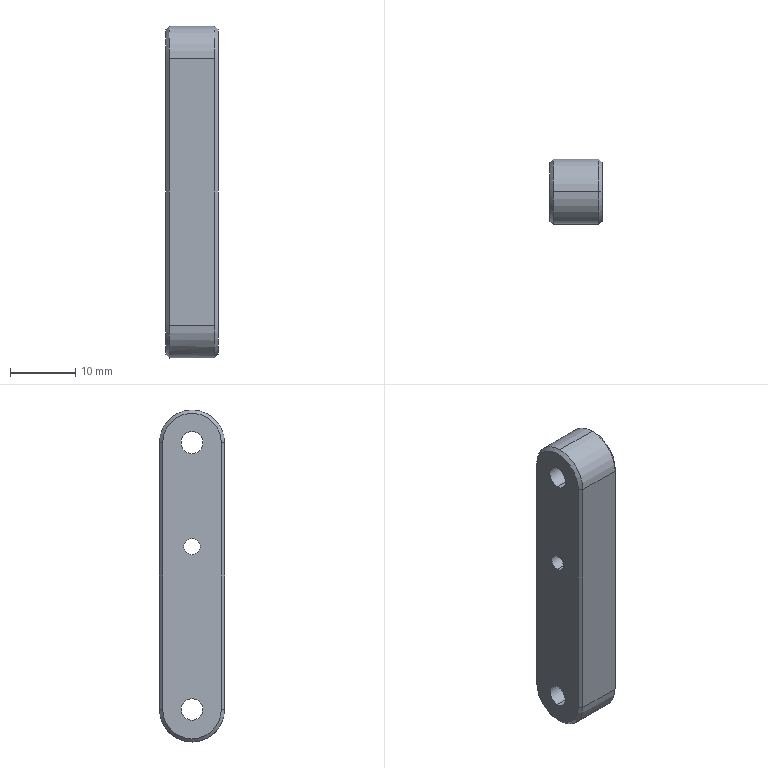Part | SolidWorks | features HoleWzd 3, Chamfer 1, Extrusion 1 | 1 solid | 26 faces | box 8 x 10 x 51 mm | volume 3618 mm3 | cylinder 11 | plane 9 | cone 6 | commonest cylinder face diameters 10 x3 2.5 x2 3.3 x2 3.4 x2 6.5 x2
STEP:
#1=CARTESIAN_POINT('',(4.,0.,25.));
#2=VERTEX_POINT('',#1);
#3=CARTESIAN_POINT('',(4.,-4.5,20.5));
#4=VERTEX_POINT('',#3);
#5=CARTESIAN_POINT('',(4.,0.,20.5));
#6=DIRECTION('',(1.,0.,0.));
#7=DIRECTION('',(0.,0.,-1.));
#8=AXIS2_PLACEMENT_3D('',#5,#6,#7);
#9=CIRCLE('',#8,4.5);
#10=EDGE_CURVE('',#2,#4,#9,.T.);
#11=ORIENTED_EDGE('',*,*,#10,.F.);
#12=CARTESIAN_POINT('',(3.5,0.,25.5));
#13=VERTEX_POINT('',#12);
#14=CARTESIAN_POINT('',(4.,0.,25.));
#15=DIRECTION('',(-0.7071,0.,0.7071));
#16=VECTOR('',#15,1000.);
#17=LINE('',#14,#16);
#18=EDGE_CURVE('',#2,#13,#17,.T.);
#19=ORIENTED_EDGE('',*,*,#18,.T.);
#20=CARTESIAN_POINT('',(3.5,-5.,20.5));
#21=VERTEX_POINT('',#20);
#22=CARTESIAN_POINT('',(3.5,0.,20.5));
#23=DIRECTION('',(-1.,0.,0.));
#24=DIRECTION('',(0.,0.,-1.));
#25=AXIS2_PLACEMENT_3D('',#22,#23,#24);
#26=CIRCLE('',#25,5.);
#27=EDGE_CURVE('',#21,#13,#26,.T.);
#28=ORIENTED_EDGE('',*,*,#27,.F.);
#29=CARTESIAN_POINT('',(3.5,-5.,20.5));
#30=DIRECTION('',(0.7071,0.7071,0.));
#31=VECTOR('',#30,1000.);
#32=LINE('',#29,#31);
#33=EDGE_CURVE('',#21,#4,#32,.T.);
#34=ORIENTED_EDGE('',*,*,#33,.T.);
#35=EDGE_LOOP('',(#11,#19,#28,#34));
#36=FACE_OUTER_BOUND('',#35,.T.);
#37=CARTESIAN_POINT('',(4.,0.,20.5));
#38=DIRECTION('',(-1.,0.,0.));
#39=DIRECTION('',(0.,0.,1.));
#40=AXIS2_PLACEMENT_3D('',#37,#38,#39);
#41=CONICAL_SURFACE('',#40,4.5,0.7854);
#42=ADVANCED_FACE('',(#36),#41,.T.);
#43=CARTESIAN_POINT('',(-4.,0.,-25.));
#44=VERTEX_POINT('',#43);
#45=CARTESIAN_POINT('',(-4.,-4.5,-20.5));
#46=VERTEX_POINT('',#45);
#47=CARTESIAN_POINT('',(-4.,0.,-20.5));
#48=DIRECTION('',(-1.,0.,0.));
#49=DIRECTION('',(0.,0.,-1.));
#50=AXIS2_PLACEMENT_3D('',#47,#48,#49);
#51=CIRCLE('',#50,4.5);
#52=EDGE_CURVE('',#44,#46,#51,.T.);
#53=ORIENTED_EDGE('',*,*,#52,.F.);
#54=CARTESIAN_POINT('',(-3.5,0.,-25.5));
#55=VERTEX_POINT('',#54);
#56=CARTESIAN_POINT('',(-3.5,0.,-25.5));
#57=DIRECTION('',(0.7071,0.,-0.7071));
#58=VECTOR('',#57,1000.);
#59=LINE('',#56,#58);
#60=EDGE_CURVE('',#44,#55,#59,.T.);
#61=ORIENTED_EDGE('',*,*,#60,.T.);
#62=CARTESIAN_POINT('',(-3.5,-5.,-20.5));
#63=VERTEX_POINT('',#62);
#64=CARTESIAN_POINT('',(-3.5,0.,-20.5));
#65=DIRECTION('',(1.,0.,0.));
#66=DIRECTION('',(0.,0.,-1.));
#67=AXIS2_PLACEMENT_3D('',#64,#65,#66);
#68=CIRCLE('',#67,5.);
#69=EDGE_CURVE('',#63,#55,#68,.T.);
#70=ORIENTED_EDGE('',*,*,#69,.F.);
#71=CARTESIAN_POINT('',(-3.5,-5.,-20.5));
#72=DIRECTION('',(-0.7071,0.7071,0.));
#73=VECTOR('',#72,1000.);
#74=LINE('',#71,#73);
#75=EDGE_CURVE('',#63,#46,#74,.T.);
#76=ORIENTED_EDGE('',*,*,#75,.T.);
#77=EDGE_LOOP('',(#53,#61,#70,#76));
#78=FACE_OUTER_BOUND('',#77,.T.);
#79=CARTESIAN_POINT('',(-3.5,0.,-20.5));
#80=DIRECTION('',(1.,0.,0.));
#81=DIRECTION('',(0.,0.,-1.));
#82=AXIS2_PLACEMENT_3D('',#79,#80,#81);
#83=CONICAL_SURFACE('',#82,5.,0.7854);
#84=ADVANCED_FACE('',(#78),#83,.T.);
#85=CARTESIAN_POINT('',(-4.,0.,-18.85));
#86=VERTEX_POINT('',#85);
#87=CARTESIAN_POINT('',(-4.,0.,-22.15));
#88=VERTEX_POINT('',#87);
#89=CARTESIAN_POINT('',(-4.,0.,-20.5));
#90=DIRECTION('',(1.,0.,0.));
#91=DIRECTION('',(0.,0.,-1.));
#92=AXIS2_PLACEMENT_3D('',#89,#90,#91);
#93=CIRCLE('',#92,1.65);
#94=EDGE_CURVE('',#86,#88,#93,.T.);
#95=ORIENTED_EDGE('',*,*,#94,.F.);
#96=CARTESIAN_POINT('',(4.,0.,-18.85));
#97=VERTEX_POINT('',#96);
#98=CARTESIAN_POINT('',(4.,0.,-18.85));
#99=DIRECTION('',(1.,0.,0.));
#100=VECTOR('',#99,1000.);
#101=LINE('',#98,#100);
#102=EDGE_CURVE('',#86,#97,#101,.T.);
#103=ORIENTED_EDGE('',*,*,#102,.T.);
#104=CARTESIAN_POINT('',(4.,0.,-22.15));
#105=VERTEX_POINT('',#104);
#106=CARTESIAN_POINT('',(4.,0.,-20.5));
#107=DIRECTION('',(1.,0.,0.));
#108=DIRECTION('',(0.,0.,-1.));
#109=AXIS2_PLACEMENT_3D('',#106,#107,#108);
#110=CIRCLE('',#109,1.65);
#111=EDGE_CURVE('',#97,#105,#110,.T.);
#112=ORIENTED_EDGE('',*,*,#111,.T.);
#113=CARTESIAN_POINT('',(4.,0.,-22.15));
#114=DIRECTION('',(1.,0.,0.));
#115=VECTOR('',#114,1000.);
#116=LINE('',#113,#115);
#117=EDGE_CURVE('',#88,#105,#116,.T.);
#118=ORIENTED_EDGE('',*,*,#117,.F.);
#119=EDGE_LOOP('',(#95,#103,#112,#118));
#120=FACE_OUTER_BOUND('',#119,.T.);
#121=CARTESIAN_POINT('',(4.,0.,-20.5));
#122=DIRECTION('',(1.,0.,0.));
#123=DIRECTION('',(0.,0.,-1.));
#124=AXIS2_PLACEMENT_3D('',#121,#122,#123);
#125=CYLINDRICAL_SURFACE('',#124,1.65);
#126=ADVANCED_FACE('',(#120),#125,.F.);
#127=CARTESIAN_POINT('',(-4.,0.,5.75));
#128=VERTEX_POINT('',#127);
#129=CARTESIAN_POINT('',(-4.,0.,3.25));
#130=VERTEX_POINT('',#129);
#131=CARTESIAN_POINT('',(-4.,0.,4.5));
#132=DIRECTION('',(1.,0.,0.));
#133=DIRECTION('',(0.,0.,-1.));
#134=AXIS2_PLACEMENT_3D('',#131,#132,#133);
#135=CIRCLE('',#134,1.25);
#136=EDGE_CURVE('',#128,#130,#135,.T.);
#137=ORIENTED_EDGE('',*,*,#136,.F.);
#138=CARTESIAN_POINT('',(4.,0.,5.75));
#139=VERTEX_POINT('',#138);
#140=CARTESIAN_POINT('',(4.,0.,5.75));
#141=DIRECTION('',(1.,0.,0.));
#142=VECTOR('',#141,1000.);
#143=LINE('',#140,#142);
#144=EDGE_CURVE('',#128,#139,#143,.T.);
#145=ORIENTED_EDGE('',*,*,#144,.T.);
#146=CARTESIAN_POINT('',(4.,0.,3.25));
#147=VERTEX_POINT('',#146);
#148=CARTESIAN_POINT('',(4.,0.,4.5));
#149=DIRECTION('',(1.,0.,0.));
#150=DIRECTION('',(0.,0.,-1.));
#151=AXIS2_PLACEMENT_3D('',#148,#149,#150);
#152=CIRCLE('',#151,1.25);
#153=EDGE_CURVE('',#139,#147,#152,.T.);
#154=ORIENTED_EDGE('',*,*,#153,.T.);
#155=CARTESIAN_POINT('',(4.,0.,3.25));
#156=DIRECTION('',(1.,0.,0.));
#157=VECTOR('',#156,1000.);
#158=LINE('',#155,#157);
#159=EDGE_CURVE('',#130,#147,#158,.T.);
#160=ORIENTED_EDGE('',*,*,#159,.F.);
#161=EDGE_LOOP('',(#137,#145,#154,#160));
#162=FACE_OUTER_BOUND('',#161,.T.);
#163=CARTESIAN_POINT('',(4.,0.,4.5));
#164=DIRECTION('',(1.,0.,0.));
#165=DIRECTION('',(0.,0.,-1.));
#166=AXIS2_PLACEMENT_3D('',#163,#164,#165);
#167=CYLINDRICAL_SURFACE('',#166,1.25);
#168=ADVANCED_FACE('',(#162),#167,.F.);
#169=CARTESIAN_POINT('',(0.6,0.,23.75));
#170=VERTEX_POINT('',#169);
#171=CARTESIAN_POINT('',(0.6,0.,17.25));
#172=VERTEX_POINT('',#171);
#173=CARTESIAN_POINT('',(0.6,0.,20.5));
#174=DIRECTION('',(1.,0.,0.));
#175=DIRECTION('',(0.,0.,-1.));
#176=AXIS2_PLACEMENT_3D('',#173,#174,#175);
#177=CIRCLE('',#176,3.25);
#178=EDGE_CURVE('',#170,#172,#177,.T.);
#179=ORIENTED_EDGE('',*,*,#178,.F.);
#180=CARTESIAN_POINT('',(4.,0.,23.75));
#181=VERTEX_POINT('',#180);
#182=CARTESIAN_POINT('',(4.,0.,23.75));
#183=DIRECTION('',(1.,0.,0.));
#184=VECTOR('',#183,1000.);
#185=LINE('',#182,#184);
#186=EDGE_CURVE('',#170,#181,#185,.T.);
#187=ORIENTED_EDGE('',*,*,#186,.T.);
#188=CARTESIAN_POINT('',(4.,0.,17.25));
#189=VERTEX_POINT('',#188);
#190=CARTESIAN_POINT('',(4.,0.,20.5));
#191=DIRECTION('',(1.,0.,0.));
#192=DIRECTION('',(0.,0.,-1.));
#193=AXIS2_PLACEMENT_3D('',#190,#191,#192);
#194=CIRCLE('',#193,3.25);
#195=EDGE_CURVE('',#181,#189,#194,.T.);
#196=ORIENTED_EDGE('',*,*,#195,.T.);
#197=CARTESIAN_POINT('',(4.,0.,17.25));
#198=DIRECTION('',(1.,0.,0.));
#199=VECTOR('',#198,1000.);
#200=LINE('',#197,#199);
#201=EDGE_CURVE('',#172,#189,#200,.T.);
#202=ORIENTED_EDGE('',*,*,#201,.F.);
#203=EDGE_LOOP('',(#179,#187,#196,#202));
#204=FACE_OUTER_BOUND('',#203,.T.);
#205=CARTESIAN_POINT('',(4.,0.,20.5));
#206=DIRECTION('',(1.,0.,0.));
#207=DIRECTION('',(0.,0.,-1.));
#208=AXIS2_PLACEMENT_3D('',#205,#206,#207);
#209=CYLINDRICAL_SURFACE('',#208,3.25);
#210=ADVANCED_FACE('',(#204),#209,.F.);
#211=CARTESIAN_POINT('',(-4.,0.,22.2));
#212=VERTEX_POINT('',#211);
#213=CARTESIAN_POINT('',(-4.,0.,18.8));
#214=VERTEX_POINT('',#213);
#215=CARTESIAN_POINT('',(-4.,0.,20.5));
#216=DIRECTION('',(1.,0.,0.));
#217=DIRECTION('',(0.,0.,-1.));
#218=AXIS2_PLACEMENT_3D('',#215,#216,#217);
#219=CIRCLE('',#218,1.7);
#220=EDGE_CURVE('',#212,#214,#219,.T.);
#221=ORIENTED_EDGE('',*,*,#220,.F.);
#222=CARTESIAN_POINT('',(0.6,0.,22.2));
#223=VERTEX_POINT('',#222);
#224=CARTESIAN_POINT('',(4.,0.,22.2));
#225=DIRECTION('',(1.,0.,0.));
#226=VECTOR('',#225,1000.);
#227=LINE('',#224,#226);
#228=EDGE_CURVE('',#212,#223,#227,.T.);
#229=ORIENTED_EDGE('',*,*,#228,.T.);
#230=CARTESIAN_POINT('',(0.6,0.,18.8));
#231=VERTEX_POINT('',#230);
#232=CARTESIAN_POINT('',(0.6,0.,20.5));
#233=DIRECTION('',(1.,0.,0.));
#234=DIRECTION('',(0.,0.,-1.));
#235=AXIS2_PLACEMENT_3D('',#232,#233,#234);
#236=CIRCLE('',#235,1.7);
#237=EDGE_CURVE('',#223,#231,#236,.T.);
#238=ORIENTED_EDGE('',*,*,#237,.T.);
#239=CARTESIAN_POINT('',(4.,0.,18.8));
#240=DIRECTION('',(1.,0.,0.));
#241=VECTOR('',#240,1000.);
#242=LINE('',#239,#241);
#243=EDGE_CURVE('',#214,#231,#242,.T.);
#244=ORIENTED_EDGE('',*,*,#243,.F.);
#245=EDGE_LOOP('',(#221,#229,#238,#244));
#246=FACE_OUTER_BOUND('',#245,.T.);
#247=CARTESIAN_POINT('',(4.,0.,20.5));
#248=DIRECTION('',(1.,0.,0.));
#249=DIRECTION('',(0.,0.,-1.));
#250=AXIS2_PLACEMENT_3D('',#247,#248,#249);
#251=CYLINDRICAL_SURFACE('',#250,1.7);
#252=ADVANCED_FACE('',(#246),#251,.F.);
#253=ORIENTED_EDGE('',*,*,#27,.T.);
#254=CARTESIAN_POINT('',(-3.5,0.,25.5));
#255=VERTEX_POINT('',#254);
#256=CARTESIAN_POINT('',(4.,0.,25.5));
#257=DIRECTION('',(-1.,0.,0.));
#258=VECTOR('',#257,1000.);
#259=LINE('',#256,#258);
#260=EDGE_CURVE('',#13,#255,#259,.T.);
#261=ORIENTED_EDGE('',*,*,#260,.T.);
#262=CARTESIAN_POINT('',(-3.5,-5.,20.5));
#263=VERTEX_POINT('',#262);
#264=CARTESIAN_POINT('',(-3.5,0.,20.5));
#265=DIRECTION('',(1.,0.,0.));
#266=DIRECTION('',(0.,0.,-1.));
#267=AXIS2_PLACEMENT_3D('',#264,#265,#266);
#268=CIRCLE('',#267,5.);
#269=EDGE_CURVE('',#255,#263,#268,.T.);
#270=ORIENTED_EDGE('',*,*,#269,.T.);
#271=CARTESIAN_POINT('',(4.,-5.,20.5));
#272=DIRECTION('',(-1.,0.,0.));
#273=VECTOR('',#272,1000.);
#274=LINE('',#271,#273);
#275=EDGE_CURVE('',#21,#263,#274,.T.);
#276=ORIENTED_EDGE('',*,*,#275,.F.);
#277=EDGE_LOOP('',(#253,#261,#270,#276));
#278=FACE_OUTER_BOUND('',#277,.T.);
#279=CARTESIAN_POINT('',(4.,0.,20.5));
#280=DIRECTION('',(-1.,0.,0.));
#281=DIRECTION('',(0.,0.,1.));
#282=AXIS2_PLACEMENT_3D('',#279,#280,#281);
#283=CYLINDRICAL_SURFACE('',#282,5.);
#284=ADVANCED_FACE('',(#278),#283,.T.);
#285=CARTESIAN_POINT('',(3.5,-5.,-20.5));
#286=VERTEX_POINT('',#285);
#287=CARTESIAN_POINT('',(4.,-5.,-20.5));
#288=DIRECTION('',(-1.,0.,0.));
#289=VECTOR('',#288,1000.);
#290=LINE('',#287,#289);
#291=EDGE_CURVE('',#286,#63,#290,.T.);
#292=ORIENTED_EDGE('',*,*,#291,.T.);
#293=ORIENTED_EDGE('',*,*,#69,.T.);
#294=CARTESIAN_POINT('',(-3.5,5.,-20.5));
#295=VERTEX_POINT('',#294);
#296=CARTESIAN_POINT('',(-3.5,0.,-20.5));
#297=DIRECTION('',(1.,0.,0.));
#298=DIRECTION('',(0.,0.,-1.));
#299=AXIS2_PLACEMENT_3D('',#296,#297,#298);
#300=CIRCLE('',#299,5.);
#301=EDGE_CURVE('',#55,#295,#300,.T.);
#302=ORIENTED_EDGE('',*,*,#301,.T.);
#303=CARTESIAN_POINT('',(3.5,5.,-20.5));
#304=VERTEX_POINT('',#303);
#305=CARTESIAN_POINT('',(4.,5.,-20.5));
#306=DIRECTION('',(-1.,0.,0.));
#307=VECTOR('',#306,1000.);
#308=LINE('',#305,#307);
#309=EDGE_CURVE('',#304,#295,#308,.T.);
#310=ORIENTED_EDGE('',*,*,#309,.F.);
#311=CARTESIAN_POINT('',(3.5,0.,-20.5));
#312=DIRECTION('',(-1.,0.,0.));
#313=DIRECTION('',(0.,0.,-1.));
#314=AXIS2_PLACEMENT_3D('',#311,#312,#313);
#315=CIRCLE('',#314,5.);
#316=EDGE_CURVE('',#304,#286,#315,.T.);
#317=ORIENTED_EDGE('',*,*,#316,.T.);
#318=EDGE_LOOP('',(#292,#293,#302,#310,#317));
#319=FACE_OUTER_BOUND('',#318,.T.);
#320=CARTESIAN_POINT('',(4.,0.,-20.5));
#321=DIRECTION('',(-1.,0.,0.));
#322=DIRECTION('',(0.,0.,1.));
#323=AXIS2_PLACEMENT_3D('',#320,#321,#322);
#324=CYLINDRICAL_SURFACE('',#323,5.);
#325=ADVANCED_FACE('',(#319),#324,.T.);
#326=ORIENTED_EDGE('',*,*,#309,.T.);
#327=CARTESIAN_POINT('',(-3.5,5.,20.5));
#328=VERTEX_POINT('',#327);
#329=CARTESIAN_POINT('',(-3.5,5.,-20.5));
#330=DIRECTION('',(0.,0.,1.));
#331=VECTOR('',#330,1000.);
#332=LINE('',#329,#331);
#333=EDGE_CURVE('',#295,#328,#332,.T.);
#334=ORIENTED_EDGE('',*,*,#333,.T.);
#335=CARTESIAN_POINT('',(3.5,5.,20.5));
#336=VERTEX_POINT('',#335);
#337=CARTESIAN_POINT('',(4.,5.,20.5));
#338=DIRECTION('',(-1.,0.,0.));
#339=VECTOR('',#338,1000.);
#340=LINE('',#337,#339);
#341=EDGE_CURVE('',#336,#328,#340,.T.);
#342=ORIENTED_EDGE('',*,*,#341,.F.);
#343=CARTESIAN_POINT('',(3.5,5.,-20.5));
#344=DIRECTION('',(0.,0.,-1.));
#345=VECTOR('',#344,1000.);
#346=LINE('',#343,#345);
#347=EDGE_CURVE('',#336,#304,#346,.T.);
#348=ORIENTED_EDGE('',*,*,#347,.T.);
#349=EDGE_LOOP('',(#326,#334,#342,#348));
#350=FACE_OUTER_BOUND('',#349,.T.);
#351=CARTESIAN_POINT('',(4.,5.,-20.5));
#352=DIRECTION('',(0.,-1.,0.));
#353=DIRECTION('',(0.,0.,-1.));
#354=AXIS2_PLACEMENT_3D('',#351,#352,#353);
#355=PLANE('',#354);
#356=ADVANCED_FACE('',(#350),#355,.F.);
#357=ORIENTED_EDGE('',*,*,#260,.F.);
#358=CARTESIAN_POINT('',(3.5,0.,20.5));
#359=DIRECTION('',(-1.,0.,0.));
#360=DIRECTION('',(0.,0.,-1.));
#361=AXIS2_PLACEMENT_3D('',#358,#359,#360);
#362=CIRCLE('',#361,5.);
#363=EDGE_CURVE('',#13,#336,#362,.T.);
#364=ORIENTED_EDGE('',*,*,#363,.T.);
#365=ORIENTED_EDGE('',*,*,#341,.T.);
#366=CARTESIAN_POINT('',(-3.5,0.,20.5));
#367=DIRECTION('',(1.,0.,0.));
#368=DIRECTION('',(0.,0.,-1.));
#369=AXIS2_PLACEMENT_3D('',#366,#367,#368);
#370=CIRCLE('',#369,5.);
#371=EDGE_CURVE('',#328,#255,#370,.T.);
#372=ORIENTED_EDGE('',*,*,#371,.T.);
#373=EDGE_LOOP('',(#357,#364,#365,#372));
#374=FACE_OUTER_BOUND('',#373,.T.);
#375=CARTESIAN_POINT('',(4.,0.,20.5));
#376=DIRECTION('',(-1.,0.,0.));
#377=DIRECTION('',(0.,0.,1.));
#378=AXIS2_PLACEMENT_3D('',#375,#376,#377);
#379=CYLINDRICAL_SURFACE('',#378,5.);
#380=ADVANCED_FACE('',(#374),#379,.T.);
#381=ORIENTED_EDGE('',*,*,#275,.T.);
#382=CARTESIAN_POINT('',(-3.5,-5.,-20.5));
#383=DIRECTION('',(0.,0.,-1.));
#384=VECTOR('',#383,1000.);
#385=LINE('',#382,#384);
#386=EDGE_CURVE('',#263,#63,#385,.T.);
#387=ORIENTED_EDGE('',*,*,#386,.T.);
#388=ORIENTED_EDGE('',*,*,#291,.F.);
#389=CARTESIAN_POINT('',(3.5,-5.,20.5));
#390=DIRECTION('',(0.,0.,1.));
#391=VECTOR('',#390,1000.);
#392=LINE('',#389,#391);
#393=EDGE_CURVE('',#286,#21,#392,.T.);
#394=ORIENTED_EDGE('',*,*,#393,.T.);
#395=EDGE_LOOP('',(#381,#387,#388,#394));
#396=FACE_OUTER_BOUND('',#395,.T.);
#397=CARTESIAN_POINT('',(4.,-5.,-20.5));
#398=DIRECTION('',(0.,1.,0.));
#399=DIRECTION('',(0.,0.,1.));
#400=AXIS2_PLACEMENT_3D('',#397,#398,#399);
#401=PLANE('',#400);
#402=ADVANCED_FACE('',(#396),#401,.F.);
#403=CARTESIAN_POINT('',(4.,-4.5,-20.5));
#404=VERTEX_POINT('',#403);
#405=CARTESIAN_POINT('',(4.,4.5,-20.5));
#406=VERTEX_POINT('',#405);
#407=CARTESIAN_POINT('',(4.,0.,-20.5));
#408=DIRECTION('',(1.,0.,0.));
#409=DIRECTION('',(0.,0.,-1.));
#410=AXIS2_PLACEMENT_3D('',#407,#408,#409);
#411=CIRCLE('',#410,4.5);
#412=EDGE_CURVE('',#404,#406,#411,.T.);
#413=ORIENTED_EDGE('',*,*,#412,.T.);
#414=CARTESIAN_POINT('',(4.,4.5,20.5));
#415=VERTEX_POINT('',#414);
#416=CARTESIAN_POINT('',(4.,4.5,20.5));
#417=DIRECTION('',(0.,0.,1.));
#418=VECTOR('',#417,1000.);
#419=LINE('',#416,#418);
#420=EDGE_CURVE('',#406,#415,#419,.T.);
#421=ORIENTED_EDGE('',*,*,#420,.T.);
#422=CARTESIAN_POINT('',(4.,0.,20.5));
#423=DIRECTION('',(1.,0.,0.));
#424=DIRECTION('',(0.,0.,-1.));
#425=AXIS2_PLACEMENT_3D('',#422,#423,#424);
#426=CIRCLE('',#425,4.5);
#427=EDGE_CURVE('',#415,#2,#426,.T.);
#428=ORIENTED_EDGE('',*,*,#427,.T.);
#429=ORIENTED_EDGE('',*,*,#10,.T.);
#430=CARTESIAN_POINT('',(4.,-4.5,-20.5));
#431=DIRECTION('',(0.,0.,-1.));
#432=VECTOR('',#431,1000.);
#433=LINE('',#430,#432);
#434=EDGE_CURVE('',#4,#404,#433,.T.);
#435=ORIENTED_EDGE('',*,*,#434,.T.);
#436=EDGE_LOOP('',(#413,#421,#428,#429,#435));
#437=FACE_OUTER_BOUND('',#436,.T.);
#438=CARTESIAN_POINT('',(4.,0.,-20.5));
#439=DIRECTION('',(1.,0.,0.));
#440=DIRECTION('',(0.,0.,-1.));
#441=AXIS2_PLACEMENT_3D('',#438,#439,#440);
#442=CIRCLE('',#441,1.65);
#443=EDGE_CURVE('',#105,#97,#442,.T.);
#444=ORIENTED_EDGE('',*,*,#443,.F.);
#445=ORIENTED_EDGE('',*,*,#111,.F.);
#446=EDGE_LOOP('',(#444,#445));
#447=FACE_BOUND('',#446,.T.);
#448=CARTESIAN_POINT('',(4.,0.,4.5));
#449=DIRECTION('',(1.,0.,0.));
#450=DIRECTION('',(0.,0.,-1.));
#451=AXIS2_PLACEMENT_3D('',#448,#449,#450);
#452=CIRCLE('',#451,1.25);
#453=EDGE_CURVE('',#147,#139,#452,.T.);
#454=ORIENTED_EDGE('',*,*,#453,.F.);
#455=ORIENTED_EDGE('',*,*,#153,.F.);
#456=EDGE_LOOP('',(#454,#455));
#457=FACE_BOUND('',#456,.T.);
#458=CARTESIAN_POINT('',(4.,0.,20.5));
#459=DIRECTION('',(1.,0.,0.));
#460=DIRECTION('',(0.,0.,-1.));
#461=AXIS2_PLACEMENT_3D('',#458,#459,#460);
#462=CIRCLE('',#461,3.25);
#463=EDGE_CURVE('',#189,#181,#462,.T.);
#464=ORIENTED_EDGE('',*,*,#463,.F.);
#465=ORIENTED_EDGE('',*,*,#195,.F.);
#466=EDGE_LOOP('',(#464,#465));
#467=FACE_BOUND('',#466,.T.);
#468=CARTESIAN_POINT('',(4.,0.,-20.5));
#469=DIRECTION('',(1.,0.,0.));
#470=DIRECTION('',(0.,0.,-1.));
#471=AXIS2_PLACEMENT_3D('',#468,#469,#470);
#472=PLANE('',#471);
#473=ADVANCED_FACE('',(#437,#447,#457,#467),#472,.T.);
#474=CARTESIAN_POINT('',(-4.,-4.5,20.5));
#475=VERTEX_POINT('',#474);
#476=CARTESIAN_POINT('',(-4.,4.5,20.5));
#477=VERTEX_POINT('',#476);
#478=CARTESIAN_POINT('',(-4.,0.,20.5));
#479=DIRECTION('',(-1.,0.,0.));
#480=DIRECTION('',(0.,0.,-1.));
#481=AXIS2_PLACEMENT_3D('',#478,#479,#480);
#482=CIRCLE('',#481,4.5);
#483=EDGE_CURVE('',#475,#477,#482,.T.);
#484=ORIENTED_EDGE('',*,*,#483,.T.);
#485=CARTESIAN_POINT('',(-4.,4.5,-20.5));
#486=VERTEX_POINT('',#485);
#487=CARTESIAN_POINT('',(-4.,4.5,-20.5));
#488=DIRECTION('',(0.,0.,-1.));
#489=VECTOR('',#488,1000.);
#490=LINE('',#487,#489);
#491=EDGE_CURVE('',#477,#486,#490,.T.);
#492=ORIENTED_EDGE('',*,*,#491,.T.);
#493=CARTESIAN_POINT('',(-4.,0.,-20.5));
#494=DIRECTION('',(-1.,0.,0.));
#495=DIRECTION('',(0.,0.,-1.));
#496=AXIS2_PLACEMENT_3D('',#493,#494,#495);
#497=CIRCLE('',#496,4.5);
#498=EDGE_CURVE('',#486,#44,#497,.T.);
#499=ORIENTED_EDGE('',*,*,#498,.T.);
#500=ORIENTED_EDGE('',*,*,#52,.T.);
#501=CARTESIAN_POINT('',(-4.,-4.5,-20.5));
#502=DIRECTION('',(0.,0.,1.));
#503=VECTOR('',#502,1000.);
#504=LINE('',#501,#503);
#505=EDGE_CURVE('',#46,#475,#504,.T.);
#506=ORIENTED_EDGE('',*,*,#505,.T.);
#507=EDGE_LOOP('',(#484,#492,#499,#500,#506));
#508=FACE_OUTER_BOUND('',#507,.T.);
#509=CARTESIAN_POINT('',(-4.,0.,-20.5));
#510=DIRECTION('',(1.,0.,0.));
#511=DIRECTION('',(0.,0.,-1.));
#512=AXIS2_PLACEMENT_3D('',#509,#510,#511);
#513=CIRCLE('',#512,1.65);
#514=EDGE_CURVE('',#88,#86,#513,.T.);
#515=ORIENTED_EDGE('',*,*,#514,.T.);
#516=ORIENTED_EDGE('',*,*,#94,.T.);
#517=EDGE_LOOP('',(#515,#516));
#518=FACE_BOUND('',#517,.T.);
#519=CARTESIAN_POINT('',(-4.,0.,4.5));
#520=DIRECTION('',(1.,0.,0.));
#521=DIRECTION('',(0.,0.,-1.));
#522=AXIS2_PLACEMENT_3D('',#519,#520,#521);
#523=CIRCLE('',#522,1.25);
#524=EDGE_CURVE('',#130,#128,#523,.T.);
#525=ORIENTED_EDGE('',*,*,#524,.T.);
#526=ORIENTED_EDGE('',*,*,#136,.T.);
#527=EDGE_LOOP('',(#525,#526));
#528=FACE_BOUND('',#527,.T.);
#529=CARTESIAN_POINT('',(-4.,0.,20.5));
#530=DIRECTION('',(1.,0.,0.));
#531=DIRECTION('',(0.,0.,-1.));
#532=AXIS2_PLACEMENT_3D('',#529,#530,#531);
#533=CIRCLE('',#532,1.7);
#534=EDGE_CURVE('',#214,#212,#533,.T.);
#535=ORIENTED_EDGE('',*,*,#534,.T.);
#536=ORIENTED_EDGE('',*,*,#220,.T.);
#537=EDGE_LOOP('',(#535,#536));
#538=FACE_BOUND('',#537,.T.);
#539=CARTESIAN_POINT('',(-4.,0.,-20.5));
#540=DIRECTION('',(1.,0.,0.));
#541=DIRECTION('',(0.,0.,-1.));
#542=AXIS2_PLACEMENT_3D('',#539,#540,#541);
#543=PLANE('',#542);
#544=ADVANCED_FACE('',(#508,#518,#528,#538),#543,.F.);
#545=ORIENTED_EDGE('',*,*,#228,.F.);
#546=ORIENTED_EDGE('',*,*,#534,.F.);
#547=ORIENTED_EDGE('',*,*,#243,.T.);
#548=CARTESIAN_POINT('',(0.6,0.,20.5));
#549=DIRECTION('',(1.,0.,0.));
#550=DIRECTION('',(0.,0.,-1.));
#551=AXIS2_PLACEMENT_3D('',#548,#549,#550);
#552=CIRCLE('',#551,1.7);
#553=EDGE_CURVE('',#231,#223,#552,.T.);
#554=ORIENTED_EDGE('',*,*,#553,.T.);
#555=EDGE_LOOP('',(#545,#546,#547,#554));
#556=FACE_OUTER_BOUND('',#555,.T.);
#557=CARTESIAN_POINT('',(4.,0.,20.5));
#558=DIRECTION('',(1.,0.,0.));
#559=DIRECTION('',(0.,0.,-1.));
#560=AXIS2_PLACEMENT_3D('',#557,#558,#559);
#561=CYLINDRICAL_SURFACE('',#560,1.7);
#562=ADVANCED_FACE('',(#556),#561,.F.);
#563=ORIENTED_EDGE('',*,*,#553,.F.);
#564=ORIENTED_EDGE('',*,*,#237,.F.);
#565=EDGE_LOOP('',(#563,#564));
#566=FACE_BOUND('',#565,.T.);
#567=CARTESIAN_POINT('',(0.6,0.,20.5));
#568=DIRECTION('',(1.,0.,0.));
#569=DIRECTION('',(0.,0.,-1.));
#570=AXIS2_PLACEMENT_3D('',#567,#568,#569);
#571=CIRCLE('',#570,3.25);
#572=EDGE_CURVE('',#172,#170,#571,.T.);
#573=ORIENTED_EDGE('',*,*,#572,.T.);
#574=ORIENTED_EDGE('',*,*,#178,.T.);
#575=EDGE_LOOP('',(#573,#574));
#576=FACE_OUTER_BOUND('',#575,.T.);
#577=CARTESIAN_POINT('',(0.6,1.7,20.5));
#578=DIRECTION('',(-1.,0.,0.));
#579=DIRECTION('',(0.,0.,1.));
#580=AXIS2_PLACEMENT_3D('',#577,#578,#579);
#581=PLANE('',#580);
#582=ADVANCED_FACE('',(#566,#576),#581,.F.);
#583=ORIENTED_EDGE('',*,*,#186,.F.);
#584=ORIENTED_EDGE('',*,*,#572,.F.);
#585=ORIENTED_EDGE('',*,*,#201,.T.);
#586=ORIENTED_EDGE('',*,*,#463,.T.);
#587=EDGE_LOOP('',(#583,#584,#585,#586));
#588=FACE_OUTER_BOUND('',#587,.T.);
#589=CARTESIAN_POINT('',(4.,0.,20.5));
#590=DIRECTION('',(1.,0.,0.));
#591=DIRECTION('',(0.,0.,-1.));
#592=AXIS2_PLACEMENT_3D('',#589,#590,#591);
#593=CYLINDRICAL_SURFACE('',#592,3.25);
#594=ADVANCED_FACE('',(#588),#593,.F.);
#595=ORIENTED_EDGE('',*,*,#144,.F.);
#596=ORIENTED_EDGE('',*,*,#524,.F.);
#597=ORIENTED_EDGE('',*,*,#159,.T.);
#598=ORIENTED_EDGE('',*,*,#453,.T.);
#599=EDGE_LOOP('',(#595,#596,#597,#598));
#600=FACE_OUTER_BOUND('',#599,.T.);
#601=CARTESIAN_POINT('',(4.,0.,4.5));
#602=DIRECTION('',(1.,0.,0.));
#603=DIRECTION('',(0.,0.,-1.));
#604=AXIS2_PLACEMENT_3D('',#601,#602,#603);
#605=CYLINDRICAL_SURFACE('',#604,1.25);
#606=ADVANCED_FACE('',(#600),#605,.F.);
#607=ORIENTED_EDGE('',*,*,#102,.F.);
#608=ORIENTED_EDGE('',*,*,#514,.F.);
#609=ORIENTED_EDGE('',*,*,#117,.T.);
#610=ORIENTED_EDGE('',*,*,#443,.T.);
#611=EDGE_LOOP('',(#607,#608,#609,#610));
#612=FACE_OUTER_BOUND('',#611,.T.);
#613=CARTESIAN_POINT('',(4.,0.,-20.5));
#614=DIRECTION('',(1.,0.,0.));
#615=DIRECTION('',(0.,0.,-1.));
#616=AXIS2_PLACEMENT_3D('',#613,#614,#615);
#617=CYLINDRICAL_SURFACE('',#616,1.65);
#618=ADVANCED_FACE('',(#612),#617,.F.);
#619=CARTESIAN_POINT('',(-4.,-4.5,20.5));
#620=DIRECTION('',(0.7071,-0.7071,0.));
#621=VECTOR('',#620,1000.);
#622=LINE('',#619,#621);
#623=EDGE_CURVE('',#475,#263,#622,.T.);
#624=ORIENTED_EDGE('',*,*,#623,.F.);
#625=ORIENTED_EDGE('',*,*,#505,.F.);
#626=ORIENTED_EDGE('',*,*,#75,.F.);
#627=ORIENTED_EDGE('',*,*,#386,.F.);
#628=EDGE_LOOP('',(#624,#625,#626,#627));
#629=FACE_OUTER_BOUND('',#628,.T.);
#630=CARTESIAN_POINT('',(-3.5,-5.,-20.5));
#631=DIRECTION('',(0.7071,0.7071,0.));
#632=DIRECTION('',(0.,0.,-1.));
#633=AXIS2_PLACEMENT_3D('',#630,#631,#632);
#634=PLANE('',#633);
#635=ADVANCED_FACE('',(#629),#634,.F.);
#636=ORIENTED_EDGE('',*,*,#60,.F.);
#637=ORIENTED_EDGE('',*,*,#498,.F.);
#638=CARTESIAN_POINT('',(-3.5,5.,-20.5));
#639=DIRECTION('',(-0.7071,-0.7071,0.));
#640=VECTOR('',#639,1000.);
#641=LINE('',#638,#640);
#642=EDGE_CURVE('',#295,#486,#641,.T.);
#643=ORIENTED_EDGE('',*,*,#642,.F.);
#644=ORIENTED_EDGE('',*,*,#301,.F.);
#645=EDGE_LOOP('',(#636,#637,#643,#644));
#646=FACE_OUTER_BOUND('',#645,.T.);
#647=CARTESIAN_POINT('',(-3.5,0.,-20.5));
#648=DIRECTION('',(1.,0.,0.));
#649=DIRECTION('',(0.,0.,-1.));
#650=AXIS2_PLACEMENT_3D('',#647,#648,#649);
#651=CONICAL_SURFACE('',#650,5.,0.7854);
#652=ADVANCED_FACE('',(#646),#651,.T.);
#653=ORIENTED_EDGE('',*,*,#623,.T.);
#654=ORIENTED_EDGE('',*,*,#269,.F.);
#655=ORIENTED_EDGE('',*,*,#371,.F.);
#656=CARTESIAN_POINT('',(-4.,4.5,20.5));
#657=DIRECTION('',(0.7071,0.7071,0.));
#658=VECTOR('',#657,1000.);
#659=LINE('',#656,#658);
#660=EDGE_CURVE('',#477,#328,#659,.T.);
#661=ORIENTED_EDGE('',*,*,#660,.F.);
#662=ORIENTED_EDGE('',*,*,#483,.F.);
#663=EDGE_LOOP('',(#653,#654,#655,#661,#662));
#664=FACE_OUTER_BOUND('',#663,.T.);
#665=CARTESIAN_POINT('',(-3.5,0.,20.5));
#666=DIRECTION('',(1.,0.,0.));
#667=DIRECTION('',(0.,0.,-1.));
#668=AXIS2_PLACEMENT_3D('',#665,#666,#667);
#669=CONICAL_SURFACE('',#668,5.,0.7854);
#670=ADVANCED_FACE('',(#664),#669,.T.);
#671=ORIENTED_EDGE('',*,*,#642,.T.);
#672=ORIENTED_EDGE('',*,*,#491,.F.);
#673=ORIENTED_EDGE('',*,*,#660,.T.);
#674=ORIENTED_EDGE('',*,*,#333,.F.);
#675=EDGE_LOOP('',(#671,#672,#673,#674));
#676=FACE_OUTER_BOUND('',#675,.T.);
#677=CARTESIAN_POINT('',(-3.5,5.,-20.5));
#678=DIRECTION('',(0.7071,-0.7071,0.));
#679=DIRECTION('',(0.,0.,1.));
#680=AXIS2_PLACEMENT_3D('',#677,#678,#679);
#681=PLANE('',#680);
#682=ADVANCED_FACE('',(#676),#681,.F.);
#683=ORIENTED_EDGE('',*,*,#33,.F.);
#684=ORIENTED_EDGE('',*,*,#393,.F.);
#685=CARTESIAN_POINT('',(4.,-4.5,-20.5));
#686=DIRECTION('',(-0.7071,-0.7071,0.));
#687=VECTOR('',#686,1000.);
#688=LINE('',#685,#687);
#689=EDGE_CURVE('',#404,#286,#688,.T.);
#690=ORIENTED_EDGE('',*,*,#689,.F.);
#691=ORIENTED_EDGE('',*,*,#434,.F.);
#692=EDGE_LOOP('',(#683,#684,#690,#691));
#693=FACE_OUTER_BOUND('',#692,.T.);
#694=CARTESIAN_POINT('',(4.,-4.5,-20.5));
#695=DIRECTION('',(0.7071,-0.7071,0.));
#696=DIRECTION('',(0.,0.,1.));
#697=AXIS2_PLACEMENT_3D('',#694,#695,#696);
#698=PLANE('',#697);
#699=ADVANCED_FACE('',(#693),#698,.T.);
#700=ORIENTED_EDGE('',*,*,#689,.T.);
#701=ORIENTED_EDGE('',*,*,#316,.F.);
#702=CARTESIAN_POINT('',(4.,4.5,-20.5));
#703=DIRECTION('',(-0.7071,0.7071,0.));
#704=VECTOR('',#703,1000.);
#705=LINE('',#702,#704);
#706=EDGE_CURVE('',#406,#304,#705,.T.);
#707=ORIENTED_EDGE('',*,*,#706,.F.);
#708=ORIENTED_EDGE('',*,*,#412,.F.);
#709=EDGE_LOOP('',(#700,#701,#707,#708));
#710=FACE_OUTER_BOUND('',#709,.T.);
#711=CARTESIAN_POINT('',(4.,0.,-20.5));
#712=DIRECTION('',(-1.,0.,0.));
#713=DIRECTION('',(0.,0.,1.));
#714=AXIS2_PLACEMENT_3D('',#711,#712,#713);
#715=CONICAL_SURFACE('',#714,4.5,0.7854);
#716=ADVANCED_FACE('',(#710),#715,.T.);
#717=ORIENTED_EDGE('',*,*,#18,.F.);
#718=ORIENTED_EDGE('',*,*,#427,.F.);
#719=CARTESIAN_POINT('',(3.5,5.,20.5));
#720=DIRECTION('',(0.7071,-0.7071,0.));
#721=VECTOR('',#720,1000.);
#722=LINE('',#719,#721);
#723=EDGE_CURVE('',#336,#415,#722,.T.);
#724=ORIENTED_EDGE('',*,*,#723,.F.);
#725=ORIENTED_EDGE('',*,*,#363,.F.);
#726=EDGE_LOOP('',(#717,#718,#724,#725));
#727=FACE_OUTER_BOUND('',#726,.T.);
#728=CARTESIAN_POINT('',(4.,0.,20.5));
#729=DIRECTION('',(-1.,0.,0.));
#730=DIRECTION('',(0.,0.,1.));
#731=AXIS2_PLACEMENT_3D('',#728,#729,#730);
#732=CONICAL_SURFACE('',#731,4.5,0.7854);
#733=ADVANCED_FACE('',(#727),#732,.T.);
#734=ORIENTED_EDGE('',*,*,#706,.T.);
#735=ORIENTED_EDGE('',*,*,#347,.F.);
#736=ORIENTED_EDGE('',*,*,#723,.T.);
#737=ORIENTED_EDGE('',*,*,#420,.F.);
#738=EDGE_LOOP('',(#734,#735,#736,#737));
#739=FACE_OUTER_BOUND('',#738,.T.);
#740=CARTESIAN_POINT('',(4.,4.5,-20.5));
#741=DIRECTION('',(0.7071,0.7071,0.));
#742=DIRECTION('',(0.,0.,-1.));
#743=AXIS2_PLACEMENT_3D('',#740,#741,#742);
#744=PLANE('',#743);
#745=ADVANCED_FACE('',(#739),#744,.T.);
#746=CLOSED_SHELL('',(#42,#84,#126,#168,#210,#252,#284,#325,#356,#380,#402,#473,#544,#562,#582,#594,#606,#618,#635,#652,#670,#682,#699,#716,#733,#745));
#747=MANIFOLD_SOLID_BREP('',#746);
#748=CARTESIAN_POINT('',(0.,0.,0.));
#749=DIRECTION('',(0.,0.,1.));
#750=DIRECTION('',(1.,0.,0.));
#751=AXIS2_PLACEMENT_3D('',#748,#749,#750);
#752=(LENGTH_UNIT()NAMED_UNIT(*)SI_UNIT(.MILLI.,.METRE.));
#753=UNCERTAINTY_MEASURE_WITH_UNIT(LENGTH_MEASURE(0.00001),#752,'','');
#754=(NAMED_UNIT(*)PLANE_ANGLE_UNIT()SI_UNIT($,.RADIAN.));
#755=(NAMED_UNIT(*)SI_UNIT($,.STERADIAN.)SOLID_ANGLE_UNIT());
#756=(GEOMETRIC_REPRESENTATION_CONTEXT(3)GLOBAL_UNCERTAINTY_ASSIGNED_CONTEXT((#753))GLOBAL_UNIT_ASSIGNED_CONTEXT((#752,#754,#755))REPRESENTATION_CONTEXT('',''));
#757=ADVANCED_BREP_SHAPE_REPRESENTATION('',(#747,#751),#756);